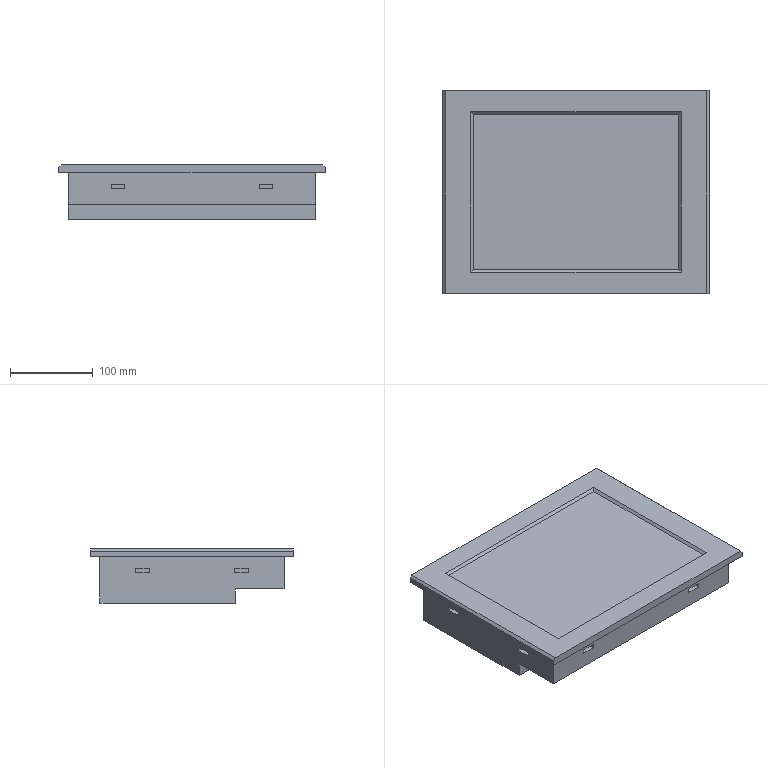Part | SolidWorks | features ICE 6, MirrorPattern 2, Chamfer 1, Extrusion 1 | 1 solid | 69 faces | box 323 x 246 x 65.5 mm | volume 4046268 mm3 | plane 65 | cylinder 4 | commonest cylinder face diameters 10 x4